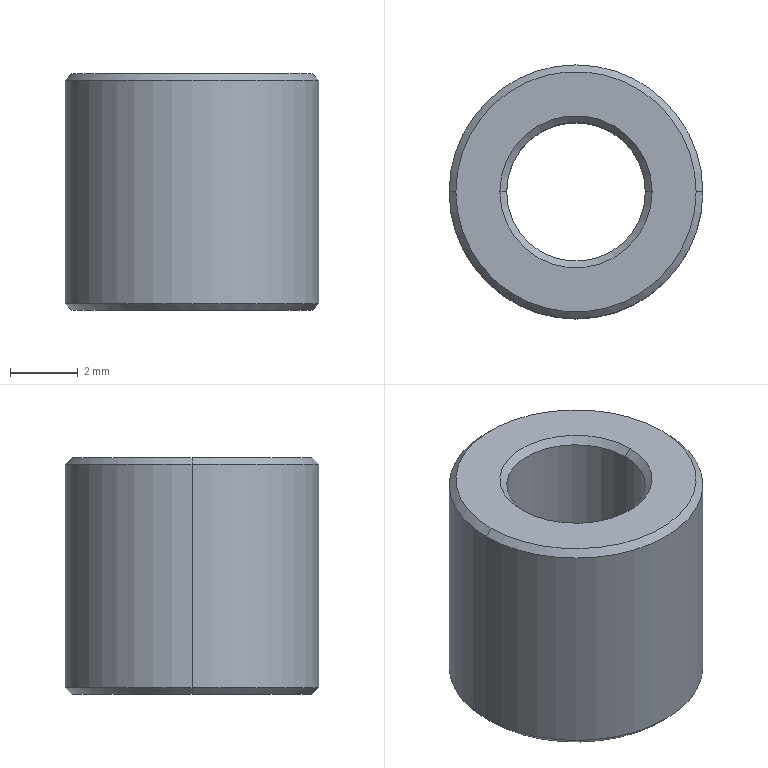Part | STEP file | 11-FG-SZ01111 | 1 solid | 14 faces | box 7.5 x 7.5 x 7 mm | volume 215.375 mm3 | cone 8 | cylinder 4 | plane 2 | commonest cylinder face diameters 4.1 x2 7.5 x2
STEP:
#1=CARTESIAN_POINT('',(-90.63,-247.716,0.));
#2=VERTEX_POINT('',#1);
#3=CARTESIAN_POINT('',(-83.53,-247.716,0.));
#4=VERTEX_POINT('',#3);
#5=CARTESIAN_POINT('',(-87.08,-247.716,0.));
#6=DIRECTION('',(0.,0.,-1.));
#7=DIRECTION('',(1.,0.,0.));
#8=AXIS2_PLACEMENT_3D('',#5,#6,#7);
#9=CIRCLE('',#8,3.55);
#10=EDGE_CURVE('',#2,#4,#9,.T.);
#11=ORIENTED_EDGE('',*,*,#10,.F.);
#12=CARTESIAN_POINT('',(-90.83,-247.716,0.2));
#13=VERTEX_POINT('',#12);
#14=CARTESIAN_POINT('',(-90.83,-247.716,0.2));
#15=DIRECTION('',(-0.7071,0.,0.7071));
#16=VECTOR('',#15,1000.);
#17=LINE('',#14,#16);
#18=EDGE_CURVE('',#2,#13,#17,.T.);
#19=ORIENTED_EDGE('',*,*,#18,.T.);
#20=CARTESIAN_POINT('',(-83.33,-247.716,0.2));
#21=VERTEX_POINT('',#20);
#22=CARTESIAN_POINT('',(-87.08,-247.716,0.2));
#23=DIRECTION('',(0.,0.,1.));
#24=DIRECTION('',(1.,0.,0.));
#25=AXIS2_PLACEMENT_3D('',#22,#23,#24);
#26=CIRCLE('',#25,3.75);
#27=EDGE_CURVE('',#21,#13,#26,.T.);
#28=ORIENTED_EDGE('',*,*,#27,.F.);
#29=CARTESIAN_POINT('',(-83.33,-247.716,0.2));
#30=DIRECTION('',(0.7071,0.,0.7071));
#31=VECTOR('',#30,1000.);
#32=LINE('',#29,#31);
#33=EDGE_CURVE('',#4,#21,#32,.T.);
#34=ORIENTED_EDGE('',*,*,#33,.F.);
#35=EDGE_LOOP('',(#11,#19,#28,#34));
#36=FACE_OUTER_BOUND('',#35,.T.);
#37=CARTESIAN_POINT('',(-87.08,-247.716,0.2));
#38=DIRECTION('',(0.,0.,1.));
#39=DIRECTION('',(1.,0.,0.));
#40=AXIS2_PLACEMENT_3D('',#37,#38,#39);
#41=CONICAL_SURFACE('',#40,3.75,0.7854);
#42=ADVANCED_FACE('',(#36),#41,.T.);
#43=CARTESIAN_POINT('',(-85.03,-247.716,0.2));
#44=VERTEX_POINT('',#43);
#45=CARTESIAN_POINT('',(-89.13,-247.716,0.2));
#46=VERTEX_POINT('',#45);
#47=CARTESIAN_POINT('',(-87.08,-247.716,0.2));
#48=DIRECTION('',(0.,0.,-1.));
#49=DIRECTION('',(1.,0.,0.));
#50=AXIS2_PLACEMENT_3D('',#47,#48,#49);
#51=CIRCLE('',#50,2.05);
#52=EDGE_CURVE('',#44,#46,#51,.T.);
#53=ORIENTED_EDGE('',*,*,#52,.F.);
#54=CARTESIAN_POINT('',(-84.83,-247.716,0.));
#55=VERTEX_POINT('',#54);
#56=CARTESIAN_POINT('',(-84.83,-247.716,0.));
#57=DIRECTION('',(0.7071,0.,-0.7071));
#58=VECTOR('',#57,1000.);
#59=LINE('',#56,#58);
#60=EDGE_CURVE('',#44,#55,#59,.T.);
#61=ORIENTED_EDGE('',*,*,#60,.T.);
#62=CARTESIAN_POINT('',(-89.33,-247.716,0.));
#63=VERTEX_POINT('',#62);
#64=CARTESIAN_POINT('',(-87.08,-247.716,0.));
#65=DIRECTION('',(0.,0.,1.));
#66=DIRECTION('',(1.,0.,0.));
#67=AXIS2_PLACEMENT_3D('',#64,#65,#66);
#68=CIRCLE('',#67,2.25);
#69=EDGE_CURVE('',#63,#55,#68,.T.);
#70=ORIENTED_EDGE('',*,*,#69,.F.);
#71=CARTESIAN_POINT('',(-89.33,-247.716,0.));
#72=DIRECTION('',(-0.7071,0.,-0.7071));
#73=VECTOR('',#72,1000.);
#74=LINE('',#71,#73);
#75=EDGE_CURVE('',#46,#63,#74,.T.);
#76=ORIENTED_EDGE('',*,*,#75,.F.);
#77=EDGE_LOOP('',(#53,#61,#70,#76));
#78=FACE_OUTER_BOUND('',#77,.T.);
#79=CARTESIAN_POINT('',(-87.08,-247.716,0.));
#80=DIRECTION('',(0.,0.,-1.));
#81=DIRECTION('',(-1.,0.,0.));
#82=AXIS2_PLACEMENT_3D('',#79,#80,#81);
#83=CONICAL_SURFACE('',#82,2.25,0.7854);
#84=ADVANCED_FACE('',(#78),#83,.F.);
#85=CARTESIAN_POINT('',(-83.53,-247.716,7.));
#86=VERTEX_POINT('',#85);
#87=CARTESIAN_POINT('',(-90.63,-247.716,7.));
#88=VERTEX_POINT('',#87);
#89=CARTESIAN_POINT('',(-87.08,-247.716,7.));
#90=DIRECTION('',(0.,0.,1.));
#91=DIRECTION('',(1.,0.,0.));
#92=AXIS2_PLACEMENT_3D('',#89,#90,#91);
#93=CIRCLE('',#92,3.55);
#94=EDGE_CURVE('',#86,#88,#93,.T.);
#95=ORIENTED_EDGE('',*,*,#94,.F.);
#96=CARTESIAN_POINT('',(-83.33,-247.716,6.8));
#97=VERTEX_POINT('',#96);
#98=CARTESIAN_POINT('',(-83.53,-247.716,7.));
#99=DIRECTION('',(0.7071,0.,-0.7071));
#100=VECTOR('',#99,1000.);
#101=LINE('',#98,#100);
#102=EDGE_CURVE('',#86,#97,#101,.T.);
#103=ORIENTED_EDGE('',*,*,#102,.T.);
#104=CARTESIAN_POINT('',(-90.83,-247.716,6.8));
#105=VERTEX_POINT('',#104);
#106=CARTESIAN_POINT('',(-87.08,-247.716,6.8));
#107=DIRECTION('',(0.,0.,-1.));
#108=DIRECTION('',(1.,0.,0.));
#109=AXIS2_PLACEMENT_3D('',#106,#107,#108);
#110=CIRCLE('',#109,3.75);
#111=EDGE_CURVE('',#105,#97,#110,.T.);
#112=ORIENTED_EDGE('',*,*,#111,.F.);
#113=CARTESIAN_POINT('',(-90.63,-247.716,7.));
#114=DIRECTION('',(-0.7071,0.,-0.7071));
#115=VECTOR('',#114,1000.);
#116=LINE('',#113,#115);
#117=EDGE_CURVE('',#88,#105,#116,.T.);
#118=ORIENTED_EDGE('',*,*,#117,.F.);
#119=EDGE_LOOP('',(#95,#103,#112,#118));
#120=FACE_OUTER_BOUND('',#119,.T.);
#121=CARTESIAN_POINT('',(-87.08,-247.716,7.));
#122=DIRECTION('',(0.,0.,-1.));
#123=DIRECTION('',(-1.,0.,0.));
#124=AXIS2_PLACEMENT_3D('',#121,#122,#123);
#125=CONICAL_SURFACE('',#124,3.55,0.7854);
#126=ADVANCED_FACE('',(#120),#125,.T.);
#127=CARTESIAN_POINT('',(-89.13,-247.716,6.8));
#128=VERTEX_POINT('',#127);
#129=CARTESIAN_POINT('',(-85.03,-247.716,6.8));
#130=VERTEX_POINT('',#129);
#131=CARTESIAN_POINT('',(-87.08,-247.716,6.8));
#132=DIRECTION('',(0.,0.,1.));
#133=DIRECTION('',(1.,0.,0.));
#134=AXIS2_PLACEMENT_3D('',#131,#132,#133);
#135=CIRCLE('',#134,2.05);
#136=EDGE_CURVE('',#128,#130,#135,.T.);
#137=ORIENTED_EDGE('',*,*,#136,.F.);
#138=CARTESIAN_POINT('',(-89.33,-247.716,7.));
#139=VERTEX_POINT('',#138);
#140=CARTESIAN_POINT('',(-89.13,-247.716,6.8));
#141=DIRECTION('',(-0.7071,0.,0.7071));
#142=VECTOR('',#141,1000.);
#143=LINE('',#140,#142);
#144=EDGE_CURVE('',#128,#139,#143,.T.);
#145=ORIENTED_EDGE('',*,*,#144,.T.);
#146=CARTESIAN_POINT('',(-84.83,-247.716,7.));
#147=VERTEX_POINT('',#146);
#148=CARTESIAN_POINT('',(-87.08,-247.716,7.));
#149=DIRECTION('',(0.,0.,-1.));
#150=DIRECTION('',(1.,0.,0.));
#151=AXIS2_PLACEMENT_3D('',#148,#149,#150);
#152=CIRCLE('',#151,2.25);
#153=EDGE_CURVE('',#147,#139,#152,.T.);
#154=ORIENTED_EDGE('',*,*,#153,.F.);
#155=CARTESIAN_POINT('',(-85.03,-247.716,6.8));
#156=DIRECTION('',(0.7071,0.,0.7071));
#157=VECTOR('',#156,1000.);
#158=LINE('',#155,#157);
#159=EDGE_CURVE('',#130,#147,#158,.T.);
#160=ORIENTED_EDGE('',*,*,#159,.F.);
#161=EDGE_LOOP('',(#137,#145,#154,#160));
#162=FACE_OUTER_BOUND('',#161,.T.);
#163=CARTESIAN_POINT('',(-87.08,-247.716,6.8));
#164=DIRECTION('',(0.,0.,1.));
#165=DIRECTION('',(1.,0.,0.));
#166=AXIS2_PLACEMENT_3D('',#163,#164,#165);
#167=CONICAL_SURFACE('',#166,2.05,0.7854);
#168=ADVANCED_FACE('',(#162),#167,.F.);
#169=ORIENTED_EDGE('',*,*,#136,.T.);
#170=CARTESIAN_POINT('',(-85.03,-247.716,7.));
#171=DIRECTION('',(0.,0.,-1.));
#172=VECTOR('',#171,1000.);
#173=LINE('',#170,#172);
#174=EDGE_CURVE('',#130,#44,#173,.T.);
#175=ORIENTED_EDGE('',*,*,#174,.T.);
#176=ORIENTED_EDGE('',*,*,#52,.T.);
#177=CARTESIAN_POINT('',(-89.13,-247.716,7.));
#178=DIRECTION('',(0.,0.,-1.));
#179=VECTOR('',#178,1000.);
#180=LINE('',#177,#179);
#181=EDGE_CURVE('',#128,#46,#180,.T.);
#182=ORIENTED_EDGE('',*,*,#181,.F.);
#183=EDGE_LOOP('',(#169,#175,#176,#182));
#184=FACE_OUTER_BOUND('',#183,.T.);
#185=CARTESIAN_POINT('',(-87.08,-247.716,7.));
#186=DIRECTION('',(0.,0.,-1.));
#187=DIRECTION('',(-1.,0.,0.));
#188=AXIS2_PLACEMENT_3D('',#185,#186,#187);
#189=CYLINDRICAL_SURFACE('',#188,2.05);
#190=ADVANCED_FACE('',(#184),#189,.F.);
#191=ORIENTED_EDGE('',*,*,#111,.T.);
#192=CARTESIAN_POINT('',(-83.33,-247.716,7.));
#193=DIRECTION('',(0.,0.,-1.));
#194=VECTOR('',#193,1000.);
#195=LINE('',#192,#194);
#196=EDGE_CURVE('',#97,#21,#195,.T.);
#197=ORIENTED_EDGE('',*,*,#196,.T.);
#198=ORIENTED_EDGE('',*,*,#27,.T.);
#199=CARTESIAN_POINT('',(-90.83,-247.716,7.));
#200=DIRECTION('',(0.,0.,-1.));
#201=VECTOR('',#200,1000.);
#202=LINE('',#199,#201);
#203=EDGE_CURVE('',#105,#13,#202,.T.);
#204=ORIENTED_EDGE('',*,*,#203,.F.);
#205=EDGE_LOOP('',(#191,#197,#198,#204));
#206=FACE_OUTER_BOUND('',#205,.T.);
#207=CARTESIAN_POINT('',(-87.08,-247.716,7.));
#208=DIRECTION('',(0.,0.,-1.));
#209=DIRECTION('',(-1.,0.,0.));
#210=AXIS2_PLACEMENT_3D('',#207,#208,#209);
#211=CYLINDRICAL_SURFACE('',#210,3.75);
#212=ADVANCED_FACE('',(#206),#211,.T.);
#213=ORIENTED_EDGE('',*,*,#153,.T.);
#214=CARTESIAN_POINT('',(-87.08,-247.716,7.));
#215=DIRECTION('',(0.,0.,-1.));
#216=DIRECTION('',(1.,0.,0.));
#217=AXIS2_PLACEMENT_3D('',#214,#215,#216);
#218=CIRCLE('',#217,2.25);
#219=EDGE_CURVE('',#139,#147,#218,.T.);
#220=ORIENTED_EDGE('',*,*,#219,.T.);
#221=EDGE_LOOP('',(#213,#220));
#222=FACE_BOUND('',#221,.T.);
#223=CARTESIAN_POINT('',(-87.08,-247.716,7.));
#224=DIRECTION('',(0.,0.,1.));
#225=DIRECTION('',(1.,0.,0.));
#226=AXIS2_PLACEMENT_3D('',#223,#224,#225);
#227=CIRCLE('',#226,3.55);
#228=EDGE_CURVE('',#88,#86,#227,.T.);
#229=ORIENTED_EDGE('',*,*,#228,.T.);
#230=ORIENTED_EDGE('',*,*,#94,.T.);
#231=EDGE_LOOP('',(#229,#230));
#232=FACE_OUTER_BOUND('',#231,.T.);
#233=CARTESIAN_POINT('',(-87.08,-247.716,7.));
#234=DIRECTION('',(0.,0.,1.));
#235=DIRECTION('',(1.,0.,0.));
#236=AXIS2_PLACEMENT_3D('',#233,#234,#235);
#237=PLANE('',#236);
#238=ADVANCED_FACE('',(#222,#232),#237,.T.);
#239=ORIENTED_EDGE('',*,*,#69,.T.);
#240=CARTESIAN_POINT('',(-87.08,-247.716,0.));
#241=DIRECTION('',(0.,0.,1.));
#242=DIRECTION('',(1.,0.,0.));
#243=AXIS2_PLACEMENT_3D('',#240,#241,#242);
#244=CIRCLE('',#243,2.25);
#245=EDGE_CURVE('',#55,#63,#244,.T.);
#246=ORIENTED_EDGE('',*,*,#245,.T.);
#247=EDGE_LOOP('',(#239,#246));
#248=FACE_BOUND('',#247,.T.);
#249=CARTESIAN_POINT('',(-87.08,-247.716,0.));
#250=DIRECTION('',(0.,0.,-1.));
#251=DIRECTION('',(1.,0.,0.));
#252=AXIS2_PLACEMENT_3D('',#249,#250,#251);
#253=CIRCLE('',#252,3.55);
#254=EDGE_CURVE('',#4,#2,#253,.T.);
#255=ORIENTED_EDGE('',*,*,#254,.T.);
#256=ORIENTED_EDGE('',*,*,#10,.T.);
#257=EDGE_LOOP('',(#255,#256));
#258=FACE_OUTER_BOUND('',#257,.T.);
#259=CARTESIAN_POINT('',(-87.08,-247.716,0.));
#260=DIRECTION('',(0.,0.,1.));
#261=DIRECTION('',(1.,0.,0.));
#262=AXIS2_PLACEMENT_3D('',#259,#260,#261);
#263=PLANE('',#262);
#264=ADVANCED_FACE('',(#248,#258),#263,.F.);
#265=ORIENTED_EDGE('',*,*,#196,.F.);
#266=CARTESIAN_POINT('',(-87.08,-247.716,6.8));
#267=DIRECTION('',(0.,0.,-1.));
#268=DIRECTION('',(1.,0.,0.));
#269=AXIS2_PLACEMENT_3D('',#266,#267,#268);
#270=CIRCLE('',#269,3.75);
#271=EDGE_CURVE('',#97,#105,#270,.T.);
#272=ORIENTED_EDGE('',*,*,#271,.T.);
#273=ORIENTED_EDGE('',*,*,#203,.T.);
#274=CARTESIAN_POINT('',(-87.08,-247.716,0.2));
#275=DIRECTION('',(0.,0.,1.));
#276=DIRECTION('',(1.,0.,0.));
#277=AXIS2_PLACEMENT_3D('',#274,#275,#276);
#278=CIRCLE('',#277,3.75);
#279=EDGE_CURVE('',#13,#21,#278,.T.);
#280=ORIENTED_EDGE('',*,*,#279,.T.);
#281=EDGE_LOOP('',(#265,#272,#273,#280));
#282=FACE_OUTER_BOUND('',#281,.T.);
#283=CARTESIAN_POINT('',(-87.08,-247.716,7.));
#284=DIRECTION('',(0.,0.,-1.));
#285=DIRECTION('',(-1.,0.,0.));
#286=AXIS2_PLACEMENT_3D('',#283,#284,#285);
#287=CYLINDRICAL_SURFACE('',#286,3.75);
#288=ADVANCED_FACE('',(#282),#287,.T.);
#289=ORIENTED_EDGE('',*,*,#174,.F.);
#290=CARTESIAN_POINT('',(-87.08,-247.716,6.8));
#291=DIRECTION('',(0.,0.,1.));
#292=DIRECTION('',(1.,0.,0.));
#293=AXIS2_PLACEMENT_3D('',#290,#291,#292);
#294=CIRCLE('',#293,2.05);
#295=EDGE_CURVE('',#130,#128,#294,.T.);
#296=ORIENTED_EDGE('',*,*,#295,.T.);
#297=ORIENTED_EDGE('',*,*,#181,.T.);
#298=CARTESIAN_POINT('',(-87.08,-247.716,0.2));
#299=DIRECTION('',(0.,0.,-1.));
#300=DIRECTION('',(1.,0.,0.));
#301=AXIS2_PLACEMENT_3D('',#298,#299,#300);
#302=CIRCLE('',#301,2.05);
#303=EDGE_CURVE('',#46,#44,#302,.T.);
#304=ORIENTED_EDGE('',*,*,#303,.T.);
#305=EDGE_LOOP('',(#289,#296,#297,#304));
#306=FACE_OUTER_BOUND('',#305,.T.);
#307=CARTESIAN_POINT('',(-87.08,-247.716,7.));
#308=DIRECTION('',(0.,0.,-1.));
#309=DIRECTION('',(-1.,0.,0.));
#310=AXIS2_PLACEMENT_3D('',#307,#308,#309);
#311=CYLINDRICAL_SURFACE('',#310,2.05);
#312=ADVANCED_FACE('',(#306),#311,.F.);
#313=ORIENTED_EDGE('',*,*,#144,.F.);
#314=ORIENTED_EDGE('',*,*,#295,.F.);
#315=ORIENTED_EDGE('',*,*,#159,.T.);
#316=ORIENTED_EDGE('',*,*,#219,.F.);
#317=EDGE_LOOP('',(#313,#314,#315,#316));
#318=FACE_OUTER_BOUND('',#317,.T.);
#319=CARTESIAN_POINT('',(-87.08,-247.716,6.8));
#320=DIRECTION('',(0.,0.,1.));
#321=DIRECTION('',(1.,0.,0.));
#322=AXIS2_PLACEMENT_3D('',#319,#320,#321);
#323=CONICAL_SURFACE('',#322,2.05,0.7854);
#324=ADVANCED_FACE('',(#318),#323,.F.);
#325=ORIENTED_EDGE('',*,*,#102,.F.);
#326=ORIENTED_EDGE('',*,*,#228,.F.);
#327=ORIENTED_EDGE('',*,*,#117,.T.);
#328=ORIENTED_EDGE('',*,*,#271,.F.);
#329=EDGE_LOOP('',(#325,#326,#327,#328));
#330=FACE_OUTER_BOUND('',#329,.T.);
#331=CARTESIAN_POINT('',(-87.08,-247.716,7.));
#332=DIRECTION('',(0.,0.,-1.));
#333=DIRECTION('',(-1.,0.,0.));
#334=AXIS2_PLACEMENT_3D('',#331,#332,#333);
#335=CONICAL_SURFACE('',#334,3.55,0.7854);
#336=ADVANCED_FACE('',(#330),#335,.T.);
#337=ORIENTED_EDGE('',*,*,#60,.F.);
#338=ORIENTED_EDGE('',*,*,#303,.F.);
#339=ORIENTED_EDGE('',*,*,#75,.T.);
#340=ORIENTED_EDGE('',*,*,#245,.F.);
#341=EDGE_LOOP('',(#337,#338,#339,#340));
#342=FACE_OUTER_BOUND('',#341,.T.);
#343=CARTESIAN_POINT('',(-87.08,-247.716,0.));
#344=DIRECTION('',(0.,0.,-1.));
#345=DIRECTION('',(-1.,0.,0.));
#346=AXIS2_PLACEMENT_3D('',#343,#344,#345);
#347=CONICAL_SURFACE('',#346,2.25,0.7854);
#348=ADVANCED_FACE('',(#342),#347,.F.);
#349=ORIENTED_EDGE('',*,*,#18,.F.);
#350=ORIENTED_EDGE('',*,*,#254,.F.);
#351=ORIENTED_EDGE('',*,*,#33,.T.);
#352=ORIENTED_EDGE('',*,*,#279,.F.);
#353=EDGE_LOOP('',(#349,#350,#351,#352));
#354=FACE_OUTER_BOUND('',#353,.T.);
#355=CARTESIAN_POINT('',(-87.08,-247.716,0.2));
#356=DIRECTION('',(0.,0.,1.));
#357=DIRECTION('',(1.,0.,0.));
#358=AXIS2_PLACEMENT_3D('',#355,#356,#357);
#359=CONICAL_SURFACE('',#358,3.75,0.7854);
#360=ADVANCED_FACE('',(#354),#359,.T.);
#361=CLOSED_SHELL('',(#42,#84,#126,#168,#190,#212,#238,#264,#288,#312,#324,#336,#348,#360));
#362=MANIFOLD_SOLID_BREP('',#361);
#363=CARTESIAN_POINT('',(0.,0.,0.));
#364=DIRECTION('',(0.,0.,1.));
#365=DIRECTION('',(1.,0.,0.));
#366=AXIS2_PLACEMENT_3D('',#363,#364,#365);
#367=(LENGTH_UNIT()NAMED_UNIT(*)SI_UNIT(.MILLI.,.METRE.));
#368=UNCERTAINTY_MEASURE_WITH_UNIT(LENGTH_MEASURE(0.00001),#367,'','');
#369=(NAMED_UNIT(*)PLANE_ANGLE_UNIT()SI_UNIT($,.RADIAN.));
#370=(NAMED_UNIT(*)SI_UNIT($,.STERADIAN.)SOLID_ANGLE_UNIT());
#371=(GEOMETRIC_REPRESENTATION_CONTEXT(3)GLOBAL_UNCERTAINTY_ASSIGNED_CONTEXT((#368))GLOBAL_UNIT_ASSIGNED_CONTEXT((#367,#369,#370))REPRESENTATION_CONTEXT('',''));
#372=ADVANCED_BREP_SHAPE_REPRESENTATION('',(#362,#366),#371);